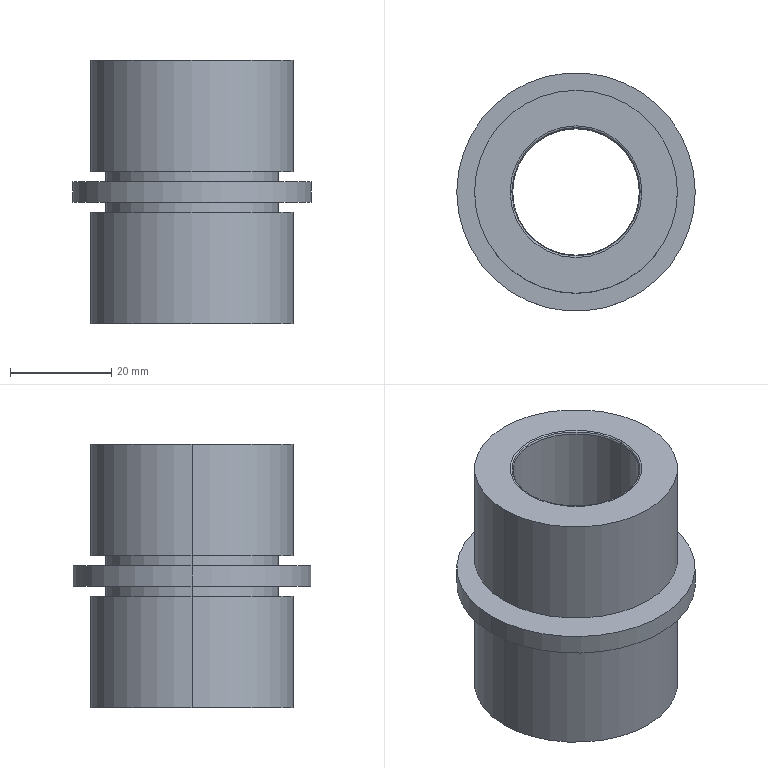Part | Creo | 1 solid | 26 faces | box 47 x 47 x 52 mm | volume 40330 mm3 | cylinder 12 | torus 8 | plane 6 | commonest cylinder face diameters 34 x4 40 x4 25 x2 47 x2
STEP:
#1=CARTESIAN_POINT('',(0.,0.,0.));
#2=DIRECTION('',(0.,0.,1.));
#3=DIRECTION('',(1.,0.,0.));
#4=AXIS2_PLACEMENT_3D('',#1,#2,#3);
#5=CARTESIAN_POINT('',(79.,141.,-253.5));
#6=VERTEX_POINT('',#5);
#7=CARTESIAN_POINT('',(119.,141.,-253.5));
#8=VERTEX_POINT('',#7);
#9=CARTESIAN_POINT('',(99.,141.,-253.5));
#10=DIRECTION('',(0.,0.,-1.));
#11=DIRECTION('',(-1.,0.,0.));
#12=AXIS2_PLACEMENT_3D('',#9,#10,#11);
#13=CIRCLE('',#12,20.);
#14=EDGE_CURVE('',#6,#8,#13,.T.);
#15=ORIENTED_EDGE('',*,*,#14,.F.);
#16=CARTESIAN_POINT('',(99.,141.,-253.5));
#17=DIRECTION('',(0.,0.,-1.));
#18=DIRECTION('',(1.,0.,0.));
#19=AXIS2_PLACEMENT_3D('',#16,#17,#18);
#20=CIRCLE('',#19,20.);
#21=EDGE_CURVE('',#8,#6,#20,.T.);
#22=ORIENTED_EDGE('',*,*,#21,.F.);
#23=EDGE_LOOP('',(#15,#22));
#24=FACE_OUTER_BOUND('',#23,.F.);
#25=CARTESIAN_POINT('',(86.,141.,-253.5));
#26=VERTEX_POINT('',#25);
#27=CARTESIAN_POINT('',(112.,141.,-253.5));
#28=VERTEX_POINT('',#27);
#29=CARTESIAN_POINT('',(99.,141.,-253.5));
#30=DIRECTION('',(0.,0.,1.));
#31=DIRECTION('',(-1.,0.,0.));
#32=AXIS2_PLACEMENT_3D('',#29,#30,#31);
#33=CIRCLE('',#32,13.);
#34=EDGE_CURVE('',#26,#28,#33,.T.);
#35=ORIENTED_EDGE('',*,*,#34,.F.);
#36=CARTESIAN_POINT('',(99.,141.,-253.5));
#37=DIRECTION('',(0.,0.,1.));
#38=DIRECTION('',(1.,0.,0.));
#39=AXIS2_PLACEMENT_3D('',#36,#37,#38);
#40=CIRCLE('',#39,13.);
#41=EDGE_CURVE('',#28,#26,#40,.T.);
#42=ORIENTED_EDGE('',*,*,#41,.F.);
#43=EDGE_LOOP('',(#35,#42));
#44=FACE_BOUND('',#43,.F.);
#45=CARTESIAN_POINT('',(99.,141.,-253.5));
#46=DIRECTION('',(0.,0.,-1.));
#47=DIRECTION('',(-1.,0.,0.));
#48=AXIS2_PLACEMENT_3D('',#45,#46,#47);
#49=PLANE('',#48);
#50=ADVANCED_FACE('',(#24,#44),#49,.T.);
#51=ORIENTED_EDGE('',*,*,#34,.T.);
#52=CARTESIAN_POINT('',(111.646,141.,-253.354));
#53=VERTEX_POINT('',#52);
#54=CARTESIAN_POINT('',(112.,141.,-253.));
#55=DIRECTION('',(0.,1.,0.));
#56=DIRECTION('',(0.,0.,-1.));
#57=AXIS2_PLACEMENT_3D('',#54,#55,#56);
#58=CIRCLE('',#57,0.5);
#59=EDGE_CURVE('',#28,#53,#58,.T.);
#60=ORIENTED_EDGE('',*,*,#59,.T.);
#61=CARTESIAN_POINT('',(86.354,141.,-253.354));
#62=VERTEX_POINT('',#61);
#63=CARTESIAN_POINT('',(99.,141.,-253.354));
#64=DIRECTION('',(0.,0.,-1.));
#65=DIRECTION('',(1.,0.,0.));
#66=AXIS2_PLACEMENT_3D('',#63,#64,#65);
#67=CIRCLE('',#66,12.646);
#68=EDGE_CURVE('',#53,#62,#67,.T.);
#69=ORIENTED_EDGE('',*,*,#68,.T.);
#70=CARTESIAN_POINT('',(86.,141.,-253.));
#71=DIRECTION('',(0.,-1.,0.));
#72=DIRECTION('',(0.,0.,-1.));
#73=AXIS2_PLACEMENT_3D('',#70,#71,#72);
#74=CIRCLE('',#73,0.5);
#75=EDGE_CURVE('',#26,#62,#74,.T.);
#76=ORIENTED_EDGE('',*,*,#75,.F.);
#77=EDGE_LOOP('',(#51,#60,#69,#76));
#78=FACE_OUTER_BOUND('',#77,.F.);
#79=CARTESIAN_POINT('',(99.,141.,-253.));
#80=DIRECTION('',(0.,0.,-1.));
#81=DIRECTION('',(1.,0.,0.));
#82=AXIS2_PLACEMENT_3D('',#79,#80,#81);
#83=TOROIDAL_SURFACE('',#82,13.,0.5);
#84=ADVANCED_FACE('',(#78),#83,.T.);
#85=ORIENTED_EDGE('',*,*,#41,.T.);
#86=ORIENTED_EDGE('',*,*,#75,.T.);
#87=CARTESIAN_POINT('',(99.,141.,-253.354));
#88=DIRECTION('',(0.,0.,-1.));
#89=DIRECTION('',(-1.,0.,0.));
#90=AXIS2_PLACEMENT_3D('',#87,#88,#89);
#91=CIRCLE('',#90,12.646);
#92=EDGE_CURVE('',#62,#53,#91,.T.);
#93=ORIENTED_EDGE('',*,*,#92,.T.);
#94=ORIENTED_EDGE('',*,*,#59,.F.);
#95=EDGE_LOOP('',(#85,#86,#93,#94));
#96=FACE_OUTER_BOUND('',#95,.F.);
#97=CARTESIAN_POINT('',(99.,141.,-253.));
#98=DIRECTION('',(0.,0.,-1.));
#99=DIRECTION('',(1.,0.,0.));
#100=AXIS2_PLACEMENT_3D('',#97,#98,#99);
#101=TOROIDAL_SURFACE('',#100,13.,0.5);
#102=ADVANCED_FACE('',(#96),#101,.T.);
#103=CARTESIAN_POINT('',(111.5,141.,-253.));
#104=VERTEX_POINT('',#103);
#105=CARTESIAN_POINT('',(86.5,141.,-253.));
#106=VERTEX_POINT('',#105);
#107=CARTESIAN_POINT('',(99.,141.,-253.));
#108=DIRECTION('',(0.,0.,1.));
#109=DIRECTION('',(1.,0.,0.));
#110=AXIS2_PLACEMENT_3D('',#107,#108,#109);
#111=CIRCLE('',#110,12.5);
#112=EDGE_CURVE('',#104,#106,#111,.T.);
#113=ORIENTED_EDGE('',*,*,#112,.F.);
#114=CARTESIAN_POINT('',(112.,141.,-253.));
#115=DIRECTION('',(0.,1.,0.));
#116=DIRECTION('',(-0.7071,0.,-0.7071));
#117=AXIS2_PLACEMENT_3D('',#114,#115,#116);
#118=CIRCLE('',#117,0.5);
#119=EDGE_CURVE('',#53,#104,#118,.T.);
#120=ORIENTED_EDGE('',*,*,#119,.F.);
#121=ORIENTED_EDGE('',*,*,#92,.F.);
#122=CARTESIAN_POINT('',(86.,141.,-253.));
#123=DIRECTION('',(0.,-1.,0.));
#124=DIRECTION('',(0.7071,0.,-0.7071));
#125=AXIS2_PLACEMENT_3D('',#122,#123,#124);
#126=CIRCLE('',#125,0.5);
#127=EDGE_CURVE('',#62,#106,#126,.T.);
#128=ORIENTED_EDGE('',*,*,#127,.T.);
#129=EDGE_LOOP('',(#113,#120,#121,#128));
#130=FACE_OUTER_BOUND('',#129,.F.);
#131=CARTESIAN_POINT('',(99.,141.,-253.));
#132=DIRECTION('',(0.,0.,-1.));
#133=DIRECTION('',(1.,0.,0.));
#134=AXIS2_PLACEMENT_3D('',#131,#132,#133);
#135=TOROIDAL_SURFACE('',#134,13.,0.5);
#136=ADVANCED_FACE('',(#130),#135,.T.);
#137=CARTESIAN_POINT('',(86.5,141.,-202.));
#138=VERTEX_POINT('',#137);
#139=CARTESIAN_POINT('',(111.5,141.,-202.));
#140=VERTEX_POINT('',#139);
#141=CARTESIAN_POINT('',(99.,141.,-202.));
#142=DIRECTION('',(0.,0.,-1.));
#143=DIRECTION('',(-1.,0.,0.));
#144=AXIS2_PLACEMENT_3D('',#141,#142,#143);
#145=CIRCLE('',#144,12.5);
#146=EDGE_CURVE('',#138,#140,#145,.T.);
#147=ORIENTED_EDGE('',*,*,#146,.T.);
#148=CARTESIAN_POINT('',(111.5,141.,-253.));
#149=DIRECTION('',(0.,0.,1.));
#150=VECTOR('',#149,51.);
#151=LINE('',#148,#150);
#152=EDGE_CURVE('',#104,#140,#151,.T.);
#153=ORIENTED_EDGE('',*,*,#152,.F.);
#154=ORIENTED_EDGE('',*,*,#112,.T.);
#155=CARTESIAN_POINT('',(86.5,141.,-253.));
#156=DIRECTION('',(0.,0.,1.));
#157=VECTOR('',#156,51.);
#158=LINE('',#155,#157);
#159=EDGE_CURVE('',#106,#138,#158,.T.);
#160=ORIENTED_EDGE('',*,*,#159,.T.);
#161=EDGE_LOOP('',(#147,#153,#154,#160));
#162=FACE_OUTER_BOUND('',#161,.F.);
#163=CARTESIAN_POINT('',(99.,141.,-253.5));
#164=DIRECTION('',(0.,0.,1.));
#165=DIRECTION('',(1.,0.,0.));
#166=AXIS2_PLACEMENT_3D('',#163,#164,#165);
#167=CYLINDRICAL_SURFACE('',#166,12.5);
#168=ADVANCED_FACE('',(#162),#167,.F.);
#169=ORIENTED_EDGE('',*,*,#146,.F.);
#170=CARTESIAN_POINT('',(86.354,141.,-201.646));
#171=VERTEX_POINT('',#170);
#172=CARTESIAN_POINT('',(86.,141.,-202.));
#173=DIRECTION('',(0.,1.,0.));
#174=DIRECTION('',(0.7071,0.,0.7071));
#175=AXIS2_PLACEMENT_3D('',#172,#173,#174);
#176=CIRCLE('',#175,0.5);
#177=EDGE_CURVE('',#171,#138,#176,.T.);
#178=ORIENTED_EDGE('',*,*,#177,.F.);
#179=CARTESIAN_POINT('',(111.646,141.,-201.646));
#180=VERTEX_POINT('',#179);
#181=CARTESIAN_POINT('',(99.,141.,-201.646));
#182=DIRECTION('',(0.,0.,1.));
#183=DIRECTION('',(1.,0.,0.));
#184=AXIS2_PLACEMENT_3D('',#181,#182,#183);
#185=CIRCLE('',#184,12.646);
#186=EDGE_CURVE('',#180,#171,#185,.T.);
#187=ORIENTED_EDGE('',*,*,#186,.F.);
#188=CARTESIAN_POINT('',(112.,141.,-202.));
#189=DIRECTION('',(0.,-1.,0.));
#190=DIRECTION('',(-0.7071,0.,0.7071));
#191=AXIS2_PLACEMENT_3D('',#188,#189,#190);
#192=CIRCLE('',#191,0.5);
#193=EDGE_CURVE('',#180,#140,#192,.T.);
#194=ORIENTED_EDGE('',*,*,#193,.T.);
#195=EDGE_LOOP('',(#169,#178,#187,#194));
#196=FACE_OUTER_BOUND('',#195,.F.);
#197=CARTESIAN_POINT('',(99.,141.,-202.));
#198=DIRECTION('',(0.,0.,1.));
#199=DIRECTION('',(-1.,0.,0.));
#200=AXIS2_PLACEMENT_3D('',#197,#198,#199);
#201=TOROIDAL_SURFACE('',#200,13.,0.5);
#202=ADVANCED_FACE('',(#196),#201,.T.);
#203=CARTESIAN_POINT('',(99.,141.,-202.));
#204=DIRECTION('',(0.,0.,-1.));
#205=DIRECTION('',(1.,0.,0.));
#206=AXIS2_PLACEMENT_3D('',#203,#204,#205);
#207=CIRCLE('',#206,12.5);
#208=EDGE_CURVE('',#140,#138,#207,.T.);
#209=ORIENTED_EDGE('',*,*,#208,.F.);
#210=ORIENTED_EDGE('',*,*,#193,.F.);
#211=CARTESIAN_POINT('',(99.,141.,-201.646));
#212=DIRECTION('',(0.,0.,1.));
#213=DIRECTION('',(-1.,0.,0.));
#214=AXIS2_PLACEMENT_3D('',#211,#212,#213);
#215=CIRCLE('',#214,12.646);
#216=EDGE_CURVE('',#171,#180,#215,.T.);
#217=ORIENTED_EDGE('',*,*,#216,.F.);
#218=ORIENTED_EDGE('',*,*,#177,.T.);
#219=EDGE_LOOP('',(#209,#210,#217,#218));
#220=FACE_OUTER_BOUND('',#219,.F.);
#221=CARTESIAN_POINT('',(99.,141.,-202.));
#222=DIRECTION('',(0.,0.,1.));
#223=DIRECTION('',(-1.,0.,0.));
#224=AXIS2_PLACEMENT_3D('',#221,#222,#223);
#225=TOROIDAL_SURFACE('',#224,13.,0.5);
#226=ADVANCED_FACE('',(#220),#225,.T.);
#227=ORIENTED_EDGE('',*,*,#208,.T.);
#228=ORIENTED_EDGE('',*,*,#159,.F.);
#229=CARTESIAN_POINT('',(99.,141.,-253.));
#230=DIRECTION('',(0.,0.,1.));
#231=DIRECTION('',(-1.,0.,0.));
#232=AXIS2_PLACEMENT_3D('',#229,#230,#231);
#233=CIRCLE('',#232,12.5);
#234=EDGE_CURVE('',#106,#104,#233,.T.);
#235=ORIENTED_EDGE('',*,*,#234,.T.);
#236=ORIENTED_EDGE('',*,*,#152,.T.);
#237=EDGE_LOOP('',(#227,#228,#235,#236));
#238=FACE_OUTER_BOUND('',#237,.F.);
#239=CARTESIAN_POINT('',(99.,141.,-253.5));
#240=DIRECTION('',(0.,0.,1.));
#241=DIRECTION('',(1.,0.,0.));
#242=AXIS2_PLACEMENT_3D('',#239,#240,#241);
#243=CYLINDRICAL_SURFACE('',#242,12.5);
#244=ADVANCED_FACE('',(#238),#243,.F.);
#245=ORIENTED_EDGE('',*,*,#234,.F.);
#246=ORIENTED_EDGE('',*,*,#127,.F.);
#247=ORIENTED_EDGE('',*,*,#68,.F.);
#248=ORIENTED_EDGE('',*,*,#119,.T.);
#249=EDGE_LOOP('',(#245,#246,#247,#248));
#250=FACE_OUTER_BOUND('',#249,.F.);
#251=CARTESIAN_POINT('',(99.,141.,-253.));
#252=DIRECTION('',(0.,0.,-1.));
#253=DIRECTION('',(1.,0.,0.));
#254=AXIS2_PLACEMENT_3D('',#251,#252,#253);
#255=TOROIDAL_SURFACE('',#254,13.,0.5);
#256=ADVANCED_FACE('',(#250),#255,.T.);
#257=CARTESIAN_POINT('',(112.,141.,-201.5));
#258=VERTEX_POINT('',#257);
#259=CARTESIAN_POINT('',(86.,141.,-201.5));
#260=VERTEX_POINT('',#259);
#261=CARTESIAN_POINT('',(99.,141.,-201.5));
#262=DIRECTION('',(0.,0.,-1.));
#263=DIRECTION('',(1.,0.,0.));
#264=AXIS2_PLACEMENT_3D('',#261,#262,#263);
#265=CIRCLE('',#264,13.);
#266=EDGE_CURVE('',#258,#260,#265,.T.);
#267=ORIENTED_EDGE('',*,*,#266,.T.);
#268=CARTESIAN_POINT('',(86.,141.,-202.));
#269=DIRECTION('',(0.,1.,0.));
#270=DIRECTION('',(0.,0.,1.));
#271=AXIS2_PLACEMENT_3D('',#268,#269,#270);
#272=CIRCLE('',#271,0.5);
#273=EDGE_CURVE('',#260,#171,#272,.T.);
#274=ORIENTED_EDGE('',*,*,#273,.T.);
#275=ORIENTED_EDGE('',*,*,#216,.T.);
#276=CARTESIAN_POINT('',(112.,141.,-202.));
#277=DIRECTION('',(0.,-1.,0.));
#278=DIRECTION('',(0.,0.,1.));
#279=AXIS2_PLACEMENT_3D('',#276,#277,#278);
#280=CIRCLE('',#279,0.5);
#281=EDGE_CURVE('',#258,#180,#280,.T.);
#282=ORIENTED_EDGE('',*,*,#281,.F.);
#283=EDGE_LOOP('',(#267,#274,#275,#282));
#284=FACE_OUTER_BOUND('',#283,.F.);
#285=CARTESIAN_POINT('',(99.,141.,-202.));
#286=DIRECTION('',(0.,0.,1.));
#287=DIRECTION('',(-1.,0.,0.));
#288=AXIS2_PLACEMENT_3D('',#285,#286,#287);
#289=TOROIDAL_SURFACE('',#288,13.,0.5);
#290=ADVANCED_FACE('',(#284),#289,.T.);
#291=CARTESIAN_POINT('',(119.,141.,-201.5));
#292=VERTEX_POINT('',#291);
#293=CARTESIAN_POINT('',(79.,141.,-201.5));
#294=VERTEX_POINT('',#293);
#295=CARTESIAN_POINT('',(99.,141.,-201.5));
#296=DIRECTION('',(0.,0.,1.));
#297=DIRECTION('',(1.,0.,0.));
#298=AXIS2_PLACEMENT_3D('',#295,#296,#297);
#299=CIRCLE('',#298,20.);
#300=EDGE_CURVE('',#292,#294,#299,.T.);
#301=ORIENTED_EDGE('',*,*,#300,.F.);
#302=CARTESIAN_POINT('',(99.,141.,-201.5));
#303=DIRECTION('',(0.,0.,1.));
#304=DIRECTION('',(-1.,0.,0.));
#305=AXIS2_PLACEMENT_3D('',#302,#303,#304);
#306=CIRCLE('',#305,20.);
#307=EDGE_CURVE('',#294,#292,#306,.T.);
#308=ORIENTED_EDGE('',*,*,#307,.F.);
#309=EDGE_LOOP('',(#301,#308));
#310=FACE_OUTER_BOUND('',#309,.F.);
#311=ORIENTED_EDGE('',*,*,#266,.F.);
#312=CARTESIAN_POINT('',(99.,141.,-201.5));
#313=DIRECTION('',(0.,0.,-1.));
#314=DIRECTION('',(-1.,0.,0.));
#315=AXIS2_PLACEMENT_3D('',#312,#313,#314);
#316=CIRCLE('',#315,13.);
#317=EDGE_CURVE('',#260,#258,#316,.T.);
#318=ORIENTED_EDGE('',*,*,#317,.F.);
#319=EDGE_LOOP('',(#311,#318));
#320=FACE_BOUND('',#319,.F.);
#321=CARTESIAN_POINT('',(99.,141.,-201.5));
#322=DIRECTION('',(0.,0.,1.));
#323=DIRECTION('',(1.,0.,0.));
#324=AXIS2_PLACEMENT_3D('',#321,#322,#323);
#325=PLANE('',#324);
#326=ADVANCED_FACE('',(#310,#320),#325,.T.);
#327=ORIENTED_EDGE('',*,*,#317,.T.);
#328=ORIENTED_EDGE('',*,*,#281,.T.);
#329=ORIENTED_EDGE('',*,*,#186,.T.);
#330=ORIENTED_EDGE('',*,*,#273,.F.);
#331=EDGE_LOOP('',(#327,#328,#329,#330));
#332=FACE_OUTER_BOUND('',#331,.F.);
#333=CARTESIAN_POINT('',(99.,141.,-202.));
#334=DIRECTION('',(0.,0.,1.));
#335=DIRECTION('',(-1.,0.,0.));
#336=AXIS2_PLACEMENT_3D('',#333,#334,#335);
#337=TOROIDAL_SURFACE('',#336,13.,0.5);
#338=ADVANCED_FACE('',(#332),#337,.T.);
#339=ORIENTED_EDGE('',*,*,#300,.T.);
#340=CARTESIAN_POINT('',(79.,141.,-223.5));
#341=VERTEX_POINT('',#340);
#342=CARTESIAN_POINT('',(79.,141.,-223.5));
#343=DIRECTION('',(0.,0.,1.));
#344=VECTOR('',#343,22.);
#345=LINE('',#342,#344);
#346=EDGE_CURVE('',#341,#294,#345,.T.);
#347=ORIENTED_EDGE('',*,*,#346,.F.);
#348=CARTESIAN_POINT('',(119.,141.,-223.5));
#349=VERTEX_POINT('',#348);
#350=CARTESIAN_POINT('',(99.,141.,-223.5));
#351=DIRECTION('',(0.,0.,-1.));
#352=DIRECTION('',(-1.,0.,0.));
#353=AXIS2_PLACEMENT_3D('',#350,#351,#352);
#354=CIRCLE('',#353,20.);
#355=EDGE_CURVE('',#341,#349,#354,.T.);
#356=ORIENTED_EDGE('',*,*,#355,.T.);
#357=CARTESIAN_POINT('',(119.,141.,-223.5));
#358=DIRECTION('',(0.,0.,1.));
#359=VECTOR('',#358,22.);
#360=LINE('',#357,#359);
#361=EDGE_CURVE('',#349,#292,#360,.T.);
#362=ORIENTED_EDGE('',*,*,#361,.T.);
#363=EDGE_LOOP('',(#339,#347,#356,#362));
#364=FACE_OUTER_BOUND('',#363,.F.);
#365=CARTESIAN_POINT('',(99.,141.,-225.5));
#366=DIRECTION('',(0.,0.,1.));
#367=DIRECTION('',(1.,0.,0.));
#368=AXIS2_PLACEMENT_3D('',#365,#366,#367);
#369=CYLINDRICAL_SURFACE('',#368,20.);
#370=ADVANCED_FACE('',(#364),#369,.T.);
#371=ORIENTED_EDGE('',*,*,#307,.T.);
#372=ORIENTED_EDGE('',*,*,#361,.F.);
#373=CARTESIAN_POINT('',(99.,141.,-223.5));
#374=DIRECTION('',(0.,0.,-1.));
#375=DIRECTION('',(1.,0.,0.));
#376=AXIS2_PLACEMENT_3D('',#373,#374,#375);
#377=CIRCLE('',#376,20.);
#378=EDGE_CURVE('',#349,#341,#377,.T.);
#379=ORIENTED_EDGE('',*,*,#378,.T.);
#380=ORIENTED_EDGE('',*,*,#346,.T.);
#381=EDGE_LOOP('',(#371,#372,#379,#380));
#382=FACE_OUTER_BOUND('',#381,.F.);
#383=CARTESIAN_POINT('',(99.,141.,-225.5));
#384=DIRECTION('',(0.,0.,1.));
#385=DIRECTION('',(1.,0.,0.));
#386=AXIS2_PLACEMENT_3D('',#383,#384,#385);
#387=CYLINDRICAL_SURFACE('',#386,20.);
#388=ADVANCED_FACE('',(#382),#387,.T.);
#389=ORIENTED_EDGE('',*,*,#378,.F.);
#390=ORIENTED_EDGE('',*,*,#355,.F.);
#391=EDGE_LOOP('',(#389,#390));
#392=FACE_OUTER_BOUND('',#391,.F.);
#393=CARTESIAN_POINT('',(116.,141.,-223.5));
#394=VERTEX_POINT('',#393);
#395=CARTESIAN_POINT('',(82.,141.,-223.5));
#396=VERTEX_POINT('',#395);
#397=CARTESIAN_POINT('',(99.,141.,-223.5));
#398=DIRECTION('',(0.,0.,1.));
#399=DIRECTION('',(1.,0.,0.));
#400=AXIS2_PLACEMENT_3D('',#397,#398,#399);
#401=CIRCLE('',#400,17.);
#402=EDGE_CURVE('',#394,#396,#401,.T.);
#403=ORIENTED_EDGE('',*,*,#402,.F.);
#404=CARTESIAN_POINT('',(99.,141.,-223.5));
#405=DIRECTION('',(0.,0.,1.));
#406=DIRECTION('',(-1.,0.,0.));
#407=AXIS2_PLACEMENT_3D('',#404,#405,#406);
#408=CIRCLE('',#407,17.);
#409=EDGE_CURVE('',#396,#394,#408,.T.);
#410=ORIENTED_EDGE('',*,*,#409,.F.);
#411=EDGE_LOOP('',(#403,#410));
#412=FACE_BOUND('',#411,.F.);
#413=CARTESIAN_POINT('',(99.,141.,-223.5));
#414=DIRECTION('',(0.,0.,1.));
#415=DIRECTION('',(-1.,0.,0.));
#416=AXIS2_PLACEMENT_3D('',#413,#414,#415);
#417=PLANE('',#416);
#418=ADVANCED_FACE('',(#392,#412),#417,.F.);
#419=ORIENTED_EDGE('',*,*,#402,.T.);
#420=CARTESIAN_POINT('',(82.,141.,-225.5));
#421=VERTEX_POINT('',#420);
#422=CARTESIAN_POINT('',(82.,141.,-225.5));
#423=DIRECTION('',(0.,0.,1.));
#424=VECTOR('',#423,2.);
#425=LINE('',#422,#424);
#426=EDGE_CURVE('',#421,#396,#425,.T.);
#427=ORIENTED_EDGE('',*,*,#426,.F.);
#428=CARTESIAN_POINT('',(116.,141.,-225.5));
#429=VERTEX_POINT('',#428);
#430=CARTESIAN_POINT('',(99.,141.,-225.5));
#431=DIRECTION('',(0.,0.,-1.));
#432=DIRECTION('',(-1.,0.,0.));
#433=AXIS2_PLACEMENT_3D('',#430,#431,#432);
#434=CIRCLE('',#433,17.);
#435=EDGE_CURVE('',#421,#429,#434,.T.);
#436=ORIENTED_EDGE('',*,*,#435,.T.);
#437=CARTESIAN_POINT('',(116.,141.,-225.5));
#438=DIRECTION('',(0.,0.,1.));
#439=VECTOR('',#438,2.);
#440=LINE('',#437,#439);
#441=EDGE_CURVE('',#429,#394,#440,.T.);
#442=ORIENTED_EDGE('',*,*,#441,.T.);
#443=EDGE_LOOP('',(#419,#427,#436,#442));
#444=FACE_OUTER_BOUND('',#443,.F.);
#445=CARTESIAN_POINT('',(99.,141.,-224.5));
#446=DIRECTION('',(0.,0.,1.));
#447=DIRECTION('',(-1.,0.,0.));
#448=AXIS2_PLACEMENT_3D('',#445,#446,#447);
#449=CYLINDRICAL_SURFACE('',#448,17.);
#450=ADVANCED_FACE('',(#444),#449,.T.);
#451=ORIENTED_EDGE('',*,*,#409,.T.);
#452=ORIENTED_EDGE('',*,*,#441,.F.);
#453=CARTESIAN_POINT('',(99.,141.,-225.5));
#454=DIRECTION('',(0.,0.,-1.));
#455=DIRECTION('',(1.,0.,0.));
#456=AXIS2_PLACEMENT_3D('',#453,#454,#455);
#457=CIRCLE('',#456,17.);
#458=EDGE_CURVE('',#429,#421,#457,.T.);
#459=ORIENTED_EDGE('',*,*,#458,.T.);
#460=ORIENTED_EDGE('',*,*,#426,.T.);
#461=EDGE_LOOP('',(#451,#452,#459,#460));
#462=FACE_OUTER_BOUND('',#461,.F.);
#463=CARTESIAN_POINT('',(99.,141.,-224.5));
#464=DIRECTION('',(0.,0.,1.));
#465=DIRECTION('',(-1.,0.,0.));
#466=AXIS2_PLACEMENT_3D('',#463,#464,#465);
#467=CYLINDRICAL_SURFACE('',#466,17.);
#468=ADVANCED_FACE('',(#462),#467,.T.);
#469=CARTESIAN_POINT('',(122.5,141.,-225.5));
#470=VERTEX_POINT('',#469);
#471=CARTESIAN_POINT('',(75.5,141.,-225.5));
#472=VERTEX_POINT('',#471);
#473=CARTESIAN_POINT('',(99.,141.,-225.5));
#474=DIRECTION('',(0.,0.,1.));
#475=DIRECTION('',(1.,0.,0.));
#476=AXIS2_PLACEMENT_3D('',#473,#474,#475);
#477=CIRCLE('',#476,23.5);
#478=EDGE_CURVE('',#470,#472,#477,.T.);
#479=ORIENTED_EDGE('',*,*,#478,.F.);
#480=CARTESIAN_POINT('',(99.,141.,-225.5));
#481=DIRECTION('',(0.,0.,1.));
#482=DIRECTION('',(-1.,0.,0.));
#483=AXIS2_PLACEMENT_3D('',#480,#481,#482);
#484=CIRCLE('',#483,23.5);
#485=EDGE_CURVE('',#472,#470,#484,.T.);
#486=ORIENTED_EDGE('',*,*,#485,.F.);
#487=EDGE_LOOP('',(#479,#486));
#488=FACE_OUTER_BOUND('',#487,.F.);
#489=ORIENTED_EDGE('',*,*,#458,.F.);
#490=ORIENTED_EDGE('',*,*,#435,.F.);
#491=EDGE_LOOP('',(#489,#490));
#492=FACE_BOUND('',#491,.F.);
#493=CARTESIAN_POINT('',(99.,141.,-225.5));
#494=DIRECTION('',(0.,0.,1.));
#495=DIRECTION('',(-1.,0.,0.));
#496=AXIS2_PLACEMENT_3D('',#493,#494,#495);
#497=PLANE('',#496);
#498=ADVANCED_FACE('',(#488,#492),#497,.T.);
#499=ORIENTED_EDGE('',*,*,#478,.T.);
#500=CARTESIAN_POINT('',(75.5,141.,-229.5));
#501=VERTEX_POINT('',#500);
#502=CARTESIAN_POINT('',(75.5,141.,-225.5));
#503=DIRECTION('',(0.,0.,-1.));
#504=VECTOR('',#503,4.);
#505=LINE('',#502,#504);
#506=EDGE_CURVE('',#472,#501,#505,.T.);
#507=ORIENTED_EDGE('',*,*,#506,.T.);
#508=CARTESIAN_POINT('',(122.5,141.,-229.5));
#509=VERTEX_POINT('',#508);
#510=CARTESIAN_POINT('',(99.,141.,-229.5));
#511=DIRECTION('',(0.,0.,-1.));
#512=DIRECTION('',(-1.,0.,0.));
#513=AXIS2_PLACEMENT_3D('',#510,#511,#512);
#514=CIRCLE('',#513,23.5);
#515=EDGE_CURVE('',#501,#509,#514,.T.);
#516=ORIENTED_EDGE('',*,*,#515,.T.);
#517=CARTESIAN_POINT('',(122.5,141.,-225.5));
#518=DIRECTION('',(0.,0.,-1.));
#519=VECTOR('',#518,4.);
#520=LINE('',#517,#519);
#521=EDGE_CURVE('',#470,#509,#520,.T.);
#522=ORIENTED_EDGE('',*,*,#521,.F.);
#523=EDGE_LOOP('',(#499,#507,#516,#522));
#524=FACE_OUTER_BOUND('',#523,.F.);
#525=CARTESIAN_POINT('',(99.,141.,-225.5));
#526=DIRECTION('',(0.,0.,-1.));
#527=DIRECTION('',(1.,0.,0.));
#528=AXIS2_PLACEMENT_3D('',#525,#526,#527);
#529=CYLINDRICAL_SURFACE('',#528,23.5);
#530=ADVANCED_FACE('',(#524),#529,.T.);
#531=ORIENTED_EDGE('',*,*,#485,.T.);
#532=ORIENTED_EDGE('',*,*,#521,.T.);
#533=CARTESIAN_POINT('',(99.,141.,-229.5));
#534=DIRECTION('',(0.,0.,-1.));
#535=DIRECTION('',(1.,0.,0.));
#536=AXIS2_PLACEMENT_3D('',#533,#534,#535);
#537=CIRCLE('',#536,23.5);
#538=EDGE_CURVE('',#509,#501,#537,.T.);
#539=ORIENTED_EDGE('',*,*,#538,.T.);
#540=ORIENTED_EDGE('',*,*,#506,.F.);
#541=EDGE_LOOP('',(#531,#532,#539,#540));
#542=FACE_OUTER_BOUND('',#541,.F.);
#543=CARTESIAN_POINT('',(99.,141.,-225.5));
#544=DIRECTION('',(0.,0.,-1.));
#545=DIRECTION('',(1.,0.,0.));
#546=AXIS2_PLACEMENT_3D('',#543,#544,#545);
#547=CYLINDRICAL_SURFACE('',#546,23.5);
#548=ADVANCED_FACE('',(#542),#547,.T.);
#549=ORIENTED_EDGE('',*,*,#538,.F.);
#550=ORIENTED_EDGE('',*,*,#515,.F.);
#551=EDGE_LOOP('',(#549,#550));
#552=FACE_OUTER_BOUND('',#551,.F.);
#553=CARTESIAN_POINT('',(82.,141.,-229.5));
#554=VERTEX_POINT('',#553);
#555=CARTESIAN_POINT('',(116.,141.,-229.5));
#556=VERTEX_POINT('',#555);
#557=CARTESIAN_POINT('',(99.,141.,-229.5));
#558=DIRECTION('',(0.,0.,1.));
#559=DIRECTION('',(-1.,0.,0.));
#560=AXIS2_PLACEMENT_3D('',#557,#558,#559);
#561=CIRCLE('',#560,17.);
#562=EDGE_CURVE('',#554,#556,#561,.T.);
#563=ORIENTED_EDGE('',*,*,#562,.F.);
#564=CARTESIAN_POINT('',(99.,141.,-229.5));
#565=DIRECTION('',(0.,0.,1.));
#566=DIRECTION('',(1.,0.,0.));
#567=AXIS2_PLACEMENT_3D('',#564,#565,#566);
#568=CIRCLE('',#567,17.);
#569=EDGE_CURVE('',#556,#554,#568,.T.);
#570=ORIENTED_EDGE('',*,*,#569,.F.);
#571=EDGE_LOOP('',(#563,#570));
#572=FACE_BOUND('',#571,.F.);
#573=CARTESIAN_POINT('',(99.,141.,-229.5));
#574=DIRECTION('',(0.,0.,1.));
#575=DIRECTION('',(-1.,0.,0.));
#576=AXIS2_PLACEMENT_3D('',#573,#574,#575);
#577=PLANE('',#576);
#578=ADVANCED_FACE('',(#552,#572),#577,.F.);
#579=CARTESIAN_POINT('',(116.,141.,-231.5));
#580=VERTEX_POINT('',#579);
#581=CARTESIAN_POINT('',(82.,141.,-231.5));
#582=VERTEX_POINT('',#581);
#583=CARTESIAN_POINT('',(99.,141.,-231.5));
#584=DIRECTION('',(0.,0.,-1.));
#585=DIRECTION('',(1.,0.,0.));
#586=AXIS2_PLACEMENT_3D('',#583,#584,#585);
#587=CIRCLE('',#586,17.);
#588=EDGE_CURVE('',#580,#582,#587,.T.);
#589=ORIENTED_EDGE('',*,*,#588,.T.);
#590=CARTESIAN_POINT('',(82.,141.,-229.5));
#591=DIRECTION('',(0.,0.,-1.));
#592=VECTOR('',#591,2.);
#593=LINE('',#590,#592);
#594=EDGE_CURVE('',#554,#582,#593,.T.);
#595=ORIENTED_EDGE('',*,*,#594,.F.);
#596=ORIENTED_EDGE('',*,*,#562,.T.);
#597=CARTESIAN_POINT('',(116.,141.,-229.5));
#598=DIRECTION('',(0.,0.,-1.));
#599=VECTOR('',#598,2.);
#600=LINE('',#597,#599);
#601=EDGE_CURVE('',#556,#580,#600,.T.);
#602=ORIENTED_EDGE('',*,*,#601,.T.);
#603=EDGE_LOOP('',(#589,#595,#596,#602));
#604=FACE_OUTER_BOUND('',#603,.F.);
#605=CARTESIAN_POINT('',(99.,141.,-230.5));
#606=DIRECTION('',(0.,0.,-1.));
#607=DIRECTION('',(1.,0.,0.));
#608=AXIS2_PLACEMENT_3D('',#605,#606,#607);
#609=CYLINDRICAL_SURFACE('',#608,17.);
#610=ADVANCED_FACE('',(#604),#609,.T.);
#611=CARTESIAN_POINT('',(79.,141.,-231.5));
#612=VERTEX_POINT('',#611);
#613=CARTESIAN_POINT('',(119.,141.,-231.5));
#614=VERTEX_POINT('',#613);
#615=CARTESIAN_POINT('',(99.,141.,-231.5));
#616=DIRECTION('',(0.,0.,1.));
#617=DIRECTION('',(-1.,0.,0.));
#618=AXIS2_PLACEMENT_3D('',#615,#616,#617);
#619=CIRCLE('',#618,20.);
#620=EDGE_CURVE('',#612,#614,#619,.T.);
#621=ORIENTED_EDGE('',*,*,#620,.F.);
#622=CARTESIAN_POINT('',(99.,141.,-231.5));
#623=DIRECTION('',(0.,0.,1.));
#624=DIRECTION('',(1.,0.,0.));
#625=AXIS2_PLACEMENT_3D('',#622,#623,#624);
#626=CIRCLE('',#625,20.);
#627=EDGE_CURVE('',#614,#612,#626,.T.);
#628=ORIENTED_EDGE('',*,*,#627,.F.);
#629=EDGE_LOOP('',(#621,#628));
#630=FACE_OUTER_BOUND('',#629,.F.);
#631=CARTESIAN_POINT('',(99.,141.,-231.5));
#632=DIRECTION('',(0.,0.,-1.));
#633=DIRECTION('',(-1.,0.,0.));
#634=AXIS2_PLACEMENT_3D('',#631,#632,#633);
#635=CIRCLE('',#634,17.);
#636=EDGE_CURVE('',#582,#580,#635,.T.);
#637=ORIENTED_EDGE('',*,*,#636,.F.);
#638=ORIENTED_EDGE('',*,*,#588,.F.);
#639=EDGE_LOOP('',(#637,#638));
#640=FACE_BOUND('',#639,.F.);
#641=CARTESIAN_POINT('',(99.,141.,-231.5));
#642=DIRECTION('',(0.,0.,-1.));
#643=DIRECTION('',(1.,0.,0.));
#644=AXIS2_PLACEMENT_3D('',#641,#642,#643);
#645=PLANE('',#644);
#646=ADVANCED_FACE('',(#630,#640),#645,.F.);
#647=ORIENTED_EDGE('',*,*,#21,.T.);
#648=CARTESIAN_POINT('',(79.,141.,-231.5));
#649=DIRECTION('',(0.,0.,-1.));
#650=VECTOR('',#649,22.);
#651=LINE('',#648,#650);
#652=EDGE_CURVE('',#612,#6,#651,.T.);
#653=ORIENTED_EDGE('',*,*,#652,.F.);
#654=ORIENTED_EDGE('',*,*,#620,.T.);
#655=CARTESIAN_POINT('',(119.,141.,-231.5));
#656=DIRECTION('',(0.,0.,-1.));
#657=VECTOR('',#656,22.);
#658=LINE('',#655,#657);
#659=EDGE_CURVE('',#614,#8,#658,.T.);
#660=ORIENTED_EDGE('',*,*,#659,.T.);
#661=EDGE_LOOP('',(#647,#653,#654,#660));
#662=FACE_OUTER_BOUND('',#661,.F.);
#663=CARTESIAN_POINT('',(99.,141.,-229.5));
#664=DIRECTION('',(0.,0.,-1.));
#665=DIRECTION('',(-1.,0.,0.));
#666=AXIS2_PLACEMENT_3D('',#663,#664,#665);
#667=CYLINDRICAL_SURFACE('',#666,20.);
#668=ADVANCED_FACE('',(#662),#667,.T.);
#669=ORIENTED_EDGE('',*,*,#14,.T.);
#670=ORIENTED_EDGE('',*,*,#659,.F.);
#671=ORIENTED_EDGE('',*,*,#627,.T.);
#672=ORIENTED_EDGE('',*,*,#652,.T.);
#673=EDGE_LOOP('',(#669,#670,#671,#672));
#674=FACE_OUTER_BOUND('',#673,.F.);
#675=CARTESIAN_POINT('',(99.,141.,-229.5));
#676=DIRECTION('',(0.,0.,-1.));
#677=DIRECTION('',(-1.,0.,0.));
#678=AXIS2_PLACEMENT_3D('',#675,#676,#677);
#679=CYLINDRICAL_SURFACE('',#678,20.);
#680=ADVANCED_FACE('',(#674),#679,.T.);
#681=ORIENTED_EDGE('',*,*,#636,.T.);
#682=ORIENTED_EDGE('',*,*,#601,.F.);
#683=ORIENTED_EDGE('',*,*,#569,.T.);
#684=ORIENTED_EDGE('',*,*,#594,.T.);
#685=EDGE_LOOP('',(#681,#682,#683,#684));
#686=FACE_OUTER_BOUND('',#685,.F.);
#687=CARTESIAN_POINT('',(99.,141.,-230.5));
#688=DIRECTION('',(0.,0.,-1.));
#689=DIRECTION('',(1.,0.,0.));
#690=AXIS2_PLACEMENT_3D('',#687,#688,#689);
#691=CYLINDRICAL_SURFACE('',#690,17.);
#692=ADVANCED_FACE('',(#686),#691,.T.);
#693=CLOSED_SHELL('',(#50,#84,#102,#136,#168,#202,#226,#244,#256,#290,#326,#338,#370,#388,#418,#450,#468,#498,#530,#548,#578,#610,#646,#668,#680,#692));
#694=MANIFOLD_SOLID_BREP('',#693);
#695=(LENGTH_UNIT()NAMED_UNIT(*)SI_UNIT(.MILLI.,.METRE.));
#696=UNCERTAINTY_MEASURE_WITH_UNIT(LENGTH_MEASURE(0.008439),#695,'','');
#697=(NAMED_UNIT(*)PLANE_ANGLE_UNIT()SI_UNIT($,.RADIAN.));
#698=PLANE_ANGLE_MEASURE_WITH_UNIT(PLANE_ANGLE_MEASURE(0.01745),#697);
#699=(CONVERSION_BASED_UNIT('DEGREE',#698)NAMED_UNIT(*)PLANE_ANGLE_UNIT());
#700=(NAMED_UNIT(*)SI_UNIT($,.STERADIAN.)SOLID_ANGLE_UNIT());
#701=(GEOMETRIC_REPRESENTATION_CONTEXT(3)GLOBAL_UNCERTAINTY_ASSIGNED_CONTEXT((#696))GLOBAL_UNIT_ASSIGNED_CONTEXT((#695,#699,#700))REPRESENTATION_CONTEXT('',''));
#702=ADVANCED_BREP_SHAPE_REPRESENTATION('',(#4,#694),#701);